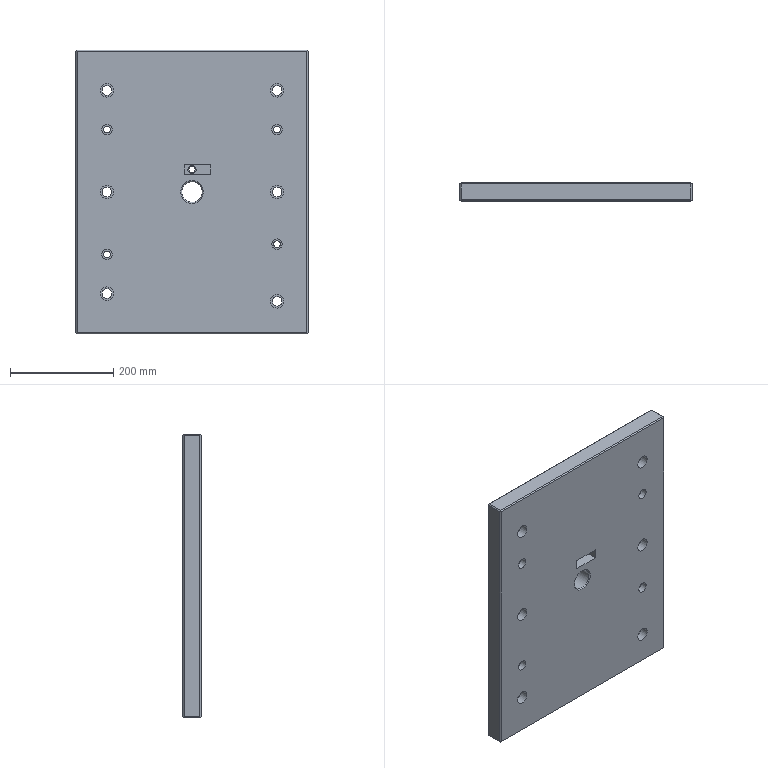Part | STEP file | BOTTOM-CLAMP-PLATE_id494_x_t | 1 solid | 59 faces | box 450 x 35 x 550 mm | volume 8473863 mm3 | plane 34 | cylinder 23 | cone 2 | commonest cylinder face diameters 18.5 x6 26 x6 13 x4 20 x4 12 x1 16 x1
STEP:
#1=CARTESIAN_POINT('',(-15.5,-265.5,53.));
#2=VERTEX_POINT('',#1);
#3=CARTESIAN_POINT('',(35.5,-265.5,53.));
#4=VERTEX_POINT('',#3);
#5=CARTESIAN_POINT('',(-15.,-265.5,53.));
#6=DIRECTION('',(1.,0.,0.));
#7=VECTOR('',#6,1.);
#8=LINE('',#5,#7);
#9=EDGE_CURVE('',#2,#4,#8,.T.);
#10=ORIENTED_EDGE('',*,*,#9,.T.);
#11=CARTESIAN_POINT('',(35.5,-290.5,53.));
#12=VERTEX_POINT('',#11);
#13=CARTESIAN_POINT('',(35.5,-290.5,53.));
#14=DIRECTION('',(0.,-1.,0.));
#15=VECTOR('',#14,1.);
#16=LINE('',#13,#15);
#17=EDGE_CURVE('',#4,#12,#16,.T.);
#18=ORIENTED_EDGE('',*,*,#17,.T.);
#19=CARTESIAN_POINT('',(-15.5,-290.5,53.));
#20=VERTEX_POINT('',#19);
#21=CARTESIAN_POINT('',(-200.,-290.5,53.));
#22=DIRECTION('',(1.,0.,0.));
#23=VECTOR('',#22,1.);
#24=LINE('',#21,#23);
#25=EDGE_CURVE('',#20,#12,#24,.T.);
#26=ORIENTED_EDGE('',*,*,#25,.F.);
#27=CARTESIAN_POINT('',(-15.5,-290.5,53.));
#28=DIRECTION('',(0.,1.,0.));
#29=VECTOR('',#28,1.);
#30=LINE('',#27,#29);
#31=EDGE_CURVE('',#20,#2,#30,.T.);
#32=ORIENTED_EDGE('',*,*,#31,.T.);
#33=EDGE_LOOP('',(#10,#18,#26,#32));
#34=FACE_OUTER_BOUND('',#33,.T.);
#35=CARTESIAN_POINT('',(35.5,-290.5,53.));
#36=DIRECTION('',(0.,0.,1.));
#37=DIRECTION('',(1.,0.,0.));
#38=AXIS2_PLACEMENT_3D('',#35,#36,#37);
#39=PLANE('',#38);
#40=ADVANCED_FACE('',(#34),#39,.F.);
#41=CARTESIAN_POINT('',(35.5,-265.5,34.));
#42=VERTEX_POINT('',#41);
#43=CARTESIAN_POINT('',(35.5,-265.5,52.5));
#44=DIRECTION('',(0.,0.,-1.));
#45=VECTOR('',#44,1.);
#46=LINE('',#43,#45);
#47=EDGE_CURVE('',#4,#42,#46,.T.);
#48=ORIENTED_EDGE('',*,*,#47,.T.);
#49=CARTESIAN_POINT('',(35.5,-290.5,34.));
#50=VERTEX_POINT('',#49);
#51=CARTESIAN_POINT('',(35.5,-290.5,34.));
#52=DIRECTION('',(0.,-1.,0.));
#53=VECTOR('',#52,1.);
#54=LINE('',#51,#53);
#55=EDGE_CURVE('',#42,#50,#54,.T.);
#56=ORIENTED_EDGE('',*,*,#55,.T.);
#57=CARTESIAN_POINT('',(35.5,-290.5,-275.));
#58=DIRECTION('',(0.,0.,-1.));
#59=VECTOR('',#58,1.);
#60=LINE('',#57,#59);
#61=EDGE_CURVE('',#12,#50,#60,.T.);
#62=ORIENTED_EDGE('',*,*,#61,.F.);
#63=ORIENTED_EDGE('',*,*,#17,.F.);
#64=EDGE_LOOP('',(#48,#56,#62,#63));
#65=FACE_OUTER_BOUND('',#64,.T.);
#66=CARTESIAN_POINT('',(35.5,-290.5,34.));
#67=DIRECTION('',(1.,0.,0.));
#68=DIRECTION('',(0.,0.,-1.));
#69=AXIS2_PLACEMENT_3D('',#66,#67,#68);
#70=PLANE('',#69);
#71=ADVANCED_FACE('',(#65),#70,.F.);
#72=CARTESIAN_POINT('',(-15.5,-265.5,34.));
#73=VERTEX_POINT('',#72);
#74=CARTESIAN_POINT('',(-15.,-265.5,34.));
#75=DIRECTION('',(-1.,0.,0.));
#76=VECTOR('',#75,1.);
#77=LINE('',#74,#76);
#78=EDGE_CURVE('',#42,#73,#77,.T.);
#79=ORIENTED_EDGE('',*,*,#78,.T.);
#80=CARTESIAN_POINT('',(-15.5,-290.5,34.));
#81=VERTEX_POINT('',#80);
#82=CARTESIAN_POINT('',(-15.5,-290.5,34.));
#83=DIRECTION('',(0.,-1.,0.));
#84=VECTOR('',#83,1.);
#85=LINE('',#82,#84);
#86=EDGE_CURVE('',#73,#81,#85,.T.);
#87=ORIENTED_EDGE('',*,*,#86,.T.);
#88=CARTESIAN_POINT('',(-200.,-290.5,34.));
#89=DIRECTION('',(-1.,0.,0.));
#90=VECTOR('',#89,1.);
#91=LINE('',#88,#90);
#92=EDGE_CURVE('',#50,#81,#91,.T.);
#93=ORIENTED_EDGE('',*,*,#92,.F.);
#94=ORIENTED_EDGE('',*,*,#55,.F.);
#95=EDGE_LOOP('',(#79,#87,#93,#94));
#96=FACE_OUTER_BOUND('',#95,.T.);
#97=CARTESIAN_POINT('',(-15.5,-290.5,34.));
#98=DIRECTION('',(0.,0.,-1.));
#99=DIRECTION('',(-1.,0.,0.));
#100=AXIS2_PLACEMENT_3D('',#97,#98,#99);
#101=PLANE('',#100);
#102=ADVANCED_FACE('',(#96),#101,.F.);
#103=CARTESIAN_POINT('',(-15.5,-265.5,52.5));
#104=DIRECTION('',(0.,0.,1.));
#105=VECTOR('',#104,1.);
#106=LINE('',#103,#105);
#107=EDGE_CURVE('',#73,#2,#106,.T.);
#108=ORIENTED_EDGE('',*,*,#107,.T.);
#109=ORIENTED_EDGE('',*,*,#31,.F.);
#110=CARTESIAN_POINT('',(-15.5,-290.5,-275.));
#111=DIRECTION('',(0.,0.,1.));
#112=VECTOR('',#111,1.);
#113=LINE('',#110,#112);
#114=EDGE_CURVE('',#81,#20,#113,.T.);
#115=ORIENTED_EDGE('',*,*,#114,.F.);
#116=ORIENTED_EDGE('',*,*,#86,.F.);
#117=EDGE_LOOP('',(#108,#109,#115,#116));
#118=FACE_OUTER_BOUND('',#117,.T.);
#119=CARTESIAN_POINT('',(-15.5,-290.5,53.));
#120=DIRECTION('',(-1.,0.,0.));
#121=DIRECTION('',(0.,0.,1.));
#122=AXIS2_PLACEMENT_3D('',#119,#120,#121);
#123=PLANE('',#122);
#124=ADVANCED_FACE('',(#118),#123,.F.);
#125=ORIENTED_EDGE('',*,*,#114,.T.);
#126=ORIENTED_EDGE('',*,*,#25,.T.);
#127=ORIENTED_EDGE('',*,*,#61,.T.);
#128=ORIENTED_EDGE('',*,*,#92,.T.);
#129=EDGE_LOOP('',(#125,#126,#127,#128));
#130=FACE_BOUND('',#129,.T.);
#131=CARTESIAN_POINT('',(-165.,-290.5,111.));
#132=VERTEX_POINT('',#131);
#133=CARTESIAN_POINT('',(-165.,-290.5,121.));
#134=DIRECTION('',(0.,1.,0.));
#135=DIRECTION('',(0.,0.,-1.));
#136=AXIS2_PLACEMENT_3D('',#133,#134,#135);
#137=CIRCLE('',#136,10.);
#138=EDGE_CURVE('',#132,#132,#137,.T.);
#139=ORIENTED_EDGE('',*,*,#138,.T.);
#140=EDGE_LOOP('',(#139));
#141=FACE_BOUND('',#140,.T.);
#142=CARTESIAN_POINT('',(165.,-290.5,111.));
#143=VERTEX_POINT('',#142);
#144=CARTESIAN_POINT('',(165.,-290.5,121.));
#145=DIRECTION('',(0.,1.,0.));
#146=DIRECTION('',(0.,0.,-1.));
#147=AXIS2_PLACEMENT_3D('',#144,#145,#146);
#148=CIRCLE('',#147,10.);
#149=EDGE_CURVE('',#143,#143,#148,.T.);
#150=ORIENTED_EDGE('',*,*,#149,.T.);
#151=EDGE_LOOP('',(#150));
#152=FACE_BOUND('',#151,.T.);
#153=CARTESIAN_POINT('',(165.,-290.5,-111.));
#154=VERTEX_POINT('',#153);
#155=CARTESIAN_POINT('',(165.,-290.5,-101.));
#156=DIRECTION('',(0.,1.,0.));
#157=DIRECTION('',(0.,0.,-1.));
#158=AXIS2_PLACEMENT_3D('',#155,#156,#157);
#159=CIRCLE('',#158,10.);
#160=EDGE_CURVE('',#154,#154,#159,.T.);
#161=ORIENTED_EDGE('',*,*,#160,.T.);
#162=EDGE_LOOP('',(#161));
#163=FACE_BOUND('',#162,.T.);
#164=CARTESIAN_POINT('',(-165.,-290.5,-131.));
#165=VERTEX_POINT('',#164);
#166=CARTESIAN_POINT('',(-165.,-290.5,-121.));
#167=DIRECTION('',(0.,1.,0.));
#168=DIRECTION('',(0.,0.,-1.));
#169=AXIS2_PLACEMENT_3D('',#166,#167,#168);
#170=CIRCLE('',#169,10.);
#171=EDGE_CURVE('',#165,#165,#170,.T.);
#172=ORIENTED_EDGE('',*,*,#171,.T.);
#173=EDGE_LOOP('',(#172));
#174=FACE_BOUND('',#173,.T.);
#175=CARTESIAN_POINT('',(165.,-290.5,-13.));
#176=VERTEX_POINT('',#175);
#177=CARTESIAN_POINT('',(165.,-290.5,0.));
#178=DIRECTION('',(0.,1.,0.));
#179=DIRECTION('',(0.,0.,-1.));
#180=AXIS2_PLACEMENT_3D('',#177,#178,#179);
#181=CIRCLE('',#180,13.);
#182=EDGE_CURVE('',#176,#176,#181,.T.);
#183=ORIENTED_EDGE('',*,*,#182,.T.);
#184=EDGE_LOOP('',(#183));
#185=FACE_BOUND('',#184,.T.);
#186=CARTESIAN_POINT('',(-165.,-290.5,-13.));
#187=VERTEX_POINT('',#186);
#188=CARTESIAN_POINT('',(-165.,-290.5,0.));
#189=DIRECTION('',(0.,1.,0.));
#190=DIRECTION('',(0.,0.,-1.));
#191=AXIS2_PLACEMENT_3D('',#188,#189,#190);
#192=CIRCLE('',#191,13.);
#193=EDGE_CURVE('',#187,#187,#192,.T.);
#194=ORIENTED_EDGE('',*,*,#193,.T.);
#195=EDGE_LOOP('',(#194));
#196=FACE_BOUND('',#195,.T.);
#197=CARTESIAN_POINT('',(-165.,-290.5,184.));
#198=VERTEX_POINT('',#197);
#199=CARTESIAN_POINT('',(-165.,-290.5,197.));
#200=DIRECTION('',(0.,1.,0.));
#201=DIRECTION('',(0.,0.,-1.));
#202=AXIS2_PLACEMENT_3D('',#199,#200,#201);
#203=CIRCLE('',#202,13.);
#204=EDGE_CURVE('',#198,#198,#203,.T.);
#205=ORIENTED_EDGE('',*,*,#204,.T.);
#206=EDGE_LOOP('',(#205));
#207=FACE_BOUND('',#206,.T.);
#208=CARTESIAN_POINT('',(165.,-290.5,184.));
#209=VERTEX_POINT('',#208);
#210=CARTESIAN_POINT('',(165.,-290.5,197.));
#211=DIRECTION('',(0.,1.,0.));
#212=DIRECTION('',(0.,0.,-1.));
#213=AXIS2_PLACEMENT_3D('',#210,#211,#212);
#214=CIRCLE('',#213,13.);
#215=EDGE_CURVE('',#209,#209,#214,.T.);
#216=ORIENTED_EDGE('',*,*,#215,.T.);
#217=EDGE_LOOP('',(#216));
#218=FACE_BOUND('',#217,.T.);
#219=CARTESIAN_POINT('',(165.,-290.5,-225.));
#220=VERTEX_POINT('',#219);
#221=CARTESIAN_POINT('',(165.,-290.5,-212.));
#222=DIRECTION('',(0.,1.,0.));
#223=DIRECTION('',(0.,0.,-1.));
#224=AXIS2_PLACEMENT_3D('',#221,#222,#223);
#225=CIRCLE('',#224,13.);
#226=EDGE_CURVE('',#220,#220,#225,.T.);
#227=ORIENTED_EDGE('',*,*,#226,.T.);
#228=EDGE_LOOP('',(#227));
#229=FACE_BOUND('',#228,.T.);
#230=CARTESIAN_POINT('',(-165.,-290.5,-210.));
#231=VERTEX_POINT('',#230);
#232=CARTESIAN_POINT('',(-165.,-290.5,-197.));
#233=DIRECTION('',(0.,1.,0.));
#234=DIRECTION('',(0.,0.,-1.));
#235=AXIS2_PLACEMENT_3D('',#232,#233,#234);
#236=CIRCLE('',#235,13.);
#237=EDGE_CURVE('',#231,#231,#236,.T.);
#238=ORIENTED_EDGE('',*,*,#237,.T.);
#239=EDGE_LOOP('',(#238));
#240=FACE_BOUND('',#239,.T.);
#241=CARTESIAN_POINT('',(0.,-290.5,-22.));
#242=VERTEX_POINT('',#241);
#243=CARTESIAN_POINT('',(0.,-290.5,0.));
#244=DIRECTION('',(0.,1.,0.));
#245=DIRECTION('',(0.,0.,-1.));
#246=AXIS2_PLACEMENT_3D('',#243,#244,#245);
#247=CIRCLE('',#246,22.);
#248=EDGE_CURVE('',#242,#242,#247,.T.);
#249=ORIENTED_EDGE('',*,*,#248,.T.);
#250=EDGE_LOOP('',(#249));
#251=FACE_BOUND('',#250,.T.);
#252=CARTESIAN_POINT('',(-223.,-290.5,-273.));
#253=VERTEX_POINT('',#252);
#254=CARTESIAN_POINT('',(223.,-290.5,-273.));
#255=VERTEX_POINT('',#254);
#256=CARTESIAN_POINT('',(-223.,-290.5,-273.));
#257=DIRECTION('',(1.,0.,0.));
#258=VECTOR('',#257,1.);
#259=LINE('',#256,#258);
#260=EDGE_CURVE('',#253,#255,#259,.T.);
#261=ORIENTED_EDGE('',*,*,#260,.T.);
#262=CARTESIAN_POINT('',(223.,-290.5,273.));
#263=VERTEX_POINT('',#262);
#264=CARTESIAN_POINT('',(223.,-290.5,-275.));
#265=DIRECTION('',(0.,0.,1.));
#266=VECTOR('',#265,1.);
#267=LINE('',#264,#266);
#268=EDGE_CURVE('',#255,#263,#267,.T.);
#269=ORIENTED_EDGE('',*,*,#268,.T.);
#270=CARTESIAN_POINT('',(-223.,-290.5,273.));
#271=VERTEX_POINT('',#270);
#272=CARTESIAN_POINT('',(223.,-290.5,273.));
#273=DIRECTION('',(-1.,0.,0.));
#274=VECTOR('',#273,1.);
#275=LINE('',#272,#274);
#276=EDGE_CURVE('',#263,#271,#275,.T.);
#277=ORIENTED_EDGE('',*,*,#276,.T.);
#278=CARTESIAN_POINT('',(-223.,-290.5,273.));
#279=DIRECTION('',(0.,0.,-1.));
#280=VECTOR('',#279,1.);
#281=LINE('',#278,#280);
#282=EDGE_CURVE('',#271,#253,#281,.T.);
#283=ORIENTED_EDGE('',*,*,#282,.T.);
#284=EDGE_LOOP('',(#261,#269,#277,#283));
#285=FACE_BOUND('',#284,.T.);
#286=CARTESIAN_POINT('',(-200.,-290.5,-275.));
#287=DIRECTION('',(0.,-1.,0.));
#288=DIRECTION('',(0.,0.,-1.));
#289=AXIS2_PLACEMENT_3D('',#286,#287,#288);
#290=PLANE('',#289);
#291=ADVANCED_FACE('',(#130,#141,#152,#163,#174,#185,#196,#207,#218,#229,#240,#251,#285),#290,.T.);
#292=CARTESIAN_POINT('',(0.,-265.5,35.5));
#293=VERTEX_POINT('',#292);
#294=CARTESIAN_POINT('',(0.,-265.5,43.5));
#295=DIRECTION('',(0.,1.,0.));
#296=DIRECTION('',(0.,0.,-1.));
#297=AXIS2_PLACEMENT_3D('',#294,#295,#296);
#298=CIRCLE('',#297,8.);
#299=EDGE_CURVE('',#293,#293,#298,.T.);
#300=ORIENTED_EDGE('',*,*,#299,.T.);
#301=EDGE_LOOP('',(#300));
#302=FACE_BOUND('',#301,.T.);
#303=ORIENTED_EDGE('',*,*,#78,.F.);
#304=ORIENTED_EDGE('',*,*,#47,.F.);
#305=ORIENTED_EDGE('',*,*,#9,.F.);
#306=ORIENTED_EDGE('',*,*,#107,.F.);
#307=EDGE_LOOP('',(#303,#304,#305,#306));
#308=FACE_BOUND('',#307,.T.);
#309=CARTESIAN_POINT('',(-15.,-265.5,52.5));
#310=DIRECTION('',(0.,1.,0.));
#311=DIRECTION('',(0.,0.,1.));
#312=AXIS2_PLACEMENT_3D('',#309,#310,#311);
#313=PLANE('',#312);
#314=ADVANCED_FACE('',(#302,#308),#313,.F.);
#315=CARTESIAN_POINT('',(225.,-288.5,-273.));
#316=VERTEX_POINT('',#315);
#317=CARTESIAN_POINT('',(224.,-289.5,-274.));
#318=VERTEX_POINT('',#317);
#319=CARTESIAN_POINT('',(225.,-288.5,-273.));
#320=DIRECTION('',(-0.5774,-0.5774,-0.5774));
#321=VECTOR('',#320,1.);
#322=LINE('',#319,#321);
#323=EDGE_CURVE('',#316,#318,#322,.T.);
#324=ORIENTED_EDGE('',*,*,#323,.F.);
#325=CARTESIAN_POINT('',(225.,-288.5,273.));
#326=VERTEX_POINT('',#325);
#327=CARTESIAN_POINT('',(225.,-288.5,-275.));
#328=DIRECTION('',(0.,0.,-1.));
#329=VECTOR('',#328,1.);
#330=LINE('',#327,#329);
#331=EDGE_CURVE('',#326,#316,#330,.T.);
#332=ORIENTED_EDGE('',*,*,#331,.F.);
#333=CARTESIAN_POINT('',(224.,-289.5,274.));
#334=VERTEX_POINT('',#333);
#335=CARTESIAN_POINT('',(224.,-289.5,274.));
#336=DIRECTION('',(0.5774,0.5774,-0.5774));
#337=VECTOR('',#336,1.);
#338=LINE('',#335,#337);
#339=EDGE_CURVE('',#334,#326,#338,.T.);
#340=ORIENTED_EDGE('',*,*,#339,.F.);
#341=CARTESIAN_POINT('',(224.,-289.5,274.));
#342=DIRECTION('',(-0.5774,-0.5774,-0.5774));
#343=VECTOR('',#342,1.);
#344=LINE('',#341,#343);
#345=EDGE_CURVE('',#334,#263,#344,.T.);
#346=ORIENTED_EDGE('',*,*,#345,.T.);
#347=ORIENTED_EDGE('',*,*,#268,.F.);
#348=CARTESIAN_POINT('',(223.,-290.5,-273.));
#349=DIRECTION('',(0.5774,0.5774,-0.5774));
#350=VECTOR('',#349,1.);
#351=LINE('',#348,#350);
#352=EDGE_CURVE('',#255,#318,#351,.T.);
#353=ORIENTED_EDGE('',*,*,#352,.T.);
#354=EDGE_LOOP('',(#324,#332,#340,#346,#347,#353));
#355=FACE_OUTER_BOUND('',#354,.T.);
#356=CARTESIAN_POINT('',(223.,-290.5,-275.));
#357=DIRECTION('',(-0.7071,0.7071,0.));
#358=DIRECTION('',(-0.7071,-0.7071,0.));
#359=AXIS2_PLACEMENT_3D('',#356,#357,#358);
#360=PLANE('',#359);
#361=ADVANCED_FACE('',(#355),#360,.F.);
#362=CARTESIAN_POINT('',(223.,-288.5,275.));
#363=VERTEX_POINT('',#362);
#364=CARTESIAN_POINT('',(223.,-288.5,275.));
#365=DIRECTION('',(0.5774,-0.5774,-0.5774));
#366=VECTOR('',#365,1.);
#367=LINE('',#364,#366);
#368=EDGE_CURVE('',#363,#334,#367,.T.);
#369=ORIENTED_EDGE('',*,*,#368,.F.);
#370=CARTESIAN_POINT('',(-223.,-288.5,275.));
#371=VERTEX_POINT('',#370);
#372=CARTESIAN_POINT('',(225.,-288.5,275.));
#373=DIRECTION('',(1.,0.,0.));
#374=VECTOR('',#373,1.);
#375=LINE('',#372,#374);
#376=EDGE_CURVE('',#371,#363,#375,.T.);
#377=ORIENTED_EDGE('',*,*,#376,.F.);
#378=CARTESIAN_POINT('',(-224.,-289.5,274.));
#379=VERTEX_POINT('',#378);
#380=CARTESIAN_POINT('',(-224.,-289.5,274.));
#381=DIRECTION('',(0.5774,0.5774,0.5774));
#382=VECTOR('',#381,1.);
#383=LINE('',#380,#382);
#384=EDGE_CURVE('',#379,#371,#383,.T.);
#385=ORIENTED_EDGE('',*,*,#384,.F.);
#386=CARTESIAN_POINT('',(-224.,-289.5,274.));
#387=DIRECTION('',(0.5774,-0.5774,-0.5774));
#388=VECTOR('',#387,1.);
#389=LINE('',#386,#388);
#390=EDGE_CURVE('',#379,#271,#389,.T.);
#391=ORIENTED_EDGE('',*,*,#390,.T.);
#392=ORIENTED_EDGE('',*,*,#276,.F.);
#393=ORIENTED_EDGE('',*,*,#345,.F.);
#394=EDGE_LOOP('',(#369,#377,#385,#391,#392,#393));
#395=FACE_OUTER_BOUND('',#394,.T.);
#396=CARTESIAN_POINT('',(223.,-290.5,273.));
#397=DIRECTION('',(0.,0.7071,-0.7071));
#398=DIRECTION('',(0.,0.7071,0.7071));
#399=AXIS2_PLACEMENT_3D('',#396,#397,#398);
#400=PLANE('',#399);
#401=ADVANCED_FACE('',(#395),#400,.F.);
#402=CARTESIAN_POINT('',(224.,-256.5,274.));
#403=VERTEX_POINT('',#402);
#404=CARTESIAN_POINT('',(223.,-257.5,275.));
#405=VERTEX_POINT('',#404);
#406=CARTESIAN_POINT('',(224.,-256.5,274.));
#407=DIRECTION('',(-0.5774,-0.5774,0.5774));
#408=VECTOR('',#407,1.);
#409=LINE('',#406,#408);
#410=EDGE_CURVE('',#403,#405,#409,.T.);
#411=ORIENTED_EDGE('',*,*,#410,.T.);
#412=CARTESIAN_POINT('',(223.,-255.5,275.));
#413=DIRECTION('',(0.,1.,0.));
#414=VECTOR('',#413,1.);
#415=LINE('',#412,#414);
#416=EDGE_CURVE('',#363,#405,#415,.T.);
#417=ORIENTED_EDGE('',*,*,#416,.F.);
#418=ORIENTED_EDGE('',*,*,#368,.T.);
#419=ORIENTED_EDGE('',*,*,#339,.T.);
#420=CARTESIAN_POINT('',(225.,-257.5,273.));
#421=VERTEX_POINT('',#420);
#422=CARTESIAN_POINT('',(225.,-255.5,273.));
#423=DIRECTION('',(0.,-1.,0.));
#424=VECTOR('',#423,1.);
#425=LINE('',#422,#424);
#426=EDGE_CURVE('',#421,#326,#425,.T.);
#427=ORIENTED_EDGE('',*,*,#426,.F.);
#428=CARTESIAN_POINT('',(225.,-257.5,273.));
#429=DIRECTION('',(-0.5774,0.5774,0.5774));
#430=VECTOR('',#429,1.);
#431=LINE('',#428,#430);
#432=EDGE_CURVE('',#421,#403,#431,.T.);
#433=ORIENTED_EDGE('',*,*,#432,.T.);
#434=EDGE_LOOP('',(#411,#417,#418,#419,#427,#433));
#435=FACE_OUTER_BOUND('',#434,.T.);
#436=CARTESIAN_POINT('',(223.,-255.5,275.));
#437=DIRECTION('',(0.7071,0.,0.7071));
#438=DIRECTION('',(0.7071,0.,-0.7071));
#439=AXIS2_PLACEMENT_3D('',#436,#437,#438);
#440=PLANE('',#439);
#441=ADVANCED_FACE('',(#435),#440,.T.);
#442=CARTESIAN_POINT('',(-225.,-288.5,273.));
#443=VERTEX_POINT('',#442);
#444=CARTESIAN_POINT('',(-225.,-288.5,273.));
#445=DIRECTION('',(0.5774,-0.5774,0.5774));
#446=VECTOR('',#445,1.);
#447=LINE('',#444,#446);
#448=EDGE_CURVE('',#443,#379,#447,.T.);
#449=ORIENTED_EDGE('',*,*,#448,.F.);
#450=CARTESIAN_POINT('',(-225.,-288.5,-273.));
#451=VERTEX_POINT('',#450);
#452=CARTESIAN_POINT('',(-225.,-288.5,275.));
#453=DIRECTION('',(0.,0.,1.));
#454=VECTOR('',#453,1.);
#455=LINE('',#452,#454);
#456=EDGE_CURVE('',#451,#443,#455,.T.);
#457=ORIENTED_EDGE('',*,*,#456,.F.);
#458=CARTESIAN_POINT('',(-224.,-289.5,-274.));
#459=VERTEX_POINT('',#458);
#460=CARTESIAN_POINT('',(-224.,-289.5,-274.));
#461=DIRECTION('',(-0.5774,0.5774,0.5774));
#462=VECTOR('',#461,1.);
#463=LINE('',#460,#462);
#464=EDGE_CURVE('',#459,#451,#463,.T.);
#465=ORIENTED_EDGE('',*,*,#464,.F.);
#466=CARTESIAN_POINT('',(-224.,-289.5,-274.));
#467=DIRECTION('',(0.5774,-0.5774,0.5774));
#468=VECTOR('',#467,1.);
#469=LINE('',#466,#468);
#470=EDGE_CURVE('',#459,#253,#469,.T.);
#471=ORIENTED_EDGE('',*,*,#470,.T.);
#472=ORIENTED_EDGE('',*,*,#282,.F.);
#473=ORIENTED_EDGE('',*,*,#390,.F.);
#474=EDGE_LOOP('',(#449,#457,#465,#471,#472,#473));
#475=FACE_OUTER_BOUND('',#474,.T.);
#476=CARTESIAN_POINT('',(-223.,-290.5,273.));
#477=DIRECTION('',(0.7071,0.7071,0.));
#478=DIRECTION('',(-0.7071,0.7071,0.));
#479=AXIS2_PLACEMENT_3D('',#476,#477,#478);
#480=PLANE('',#479);
#481=ADVANCED_FACE('',(#475),#480,.F.);
#482=CARTESIAN_POINT('',(-224.,-256.5,274.));
#483=VERTEX_POINT('',#482);
#484=CARTESIAN_POINT('',(-225.,-257.5,273.));
#485=VERTEX_POINT('',#484);
#486=CARTESIAN_POINT('',(-224.,-256.5,274.));
#487=DIRECTION('',(-0.5774,-0.5774,-0.5774));
#488=VECTOR('',#487,1.);
#489=LINE('',#486,#488);
#490=EDGE_CURVE('',#483,#485,#489,.T.);
#491=ORIENTED_EDGE('',*,*,#490,.T.);
#492=CARTESIAN_POINT('',(-225.,-255.5,273.));
#493=DIRECTION('',(0.,1.,0.));
#494=VECTOR('',#493,1.);
#495=LINE('',#492,#494);
#496=EDGE_CURVE('',#443,#485,#495,.T.);
#497=ORIENTED_EDGE('',*,*,#496,.F.);
#498=ORIENTED_EDGE('',*,*,#448,.T.);
#499=ORIENTED_EDGE('',*,*,#384,.T.);
#500=CARTESIAN_POINT('',(-223.,-257.5,275.));
#501=VERTEX_POINT('',#500);
#502=CARTESIAN_POINT('',(-223.,-255.5,275.));
#503=DIRECTION('',(0.,-1.,0.));
#504=VECTOR('',#503,1.);
#505=LINE('',#502,#504);
#506=EDGE_CURVE('',#501,#371,#505,.T.);
#507=ORIENTED_EDGE('',*,*,#506,.F.);
#508=CARTESIAN_POINT('',(-223.,-257.5,275.));
#509=DIRECTION('',(-0.5774,0.5774,-0.5774));
#510=VECTOR('',#509,1.);
#511=LINE('',#508,#510);
#512=EDGE_CURVE('',#501,#483,#511,.T.);
#513=ORIENTED_EDGE('',*,*,#512,.T.);
#514=EDGE_LOOP('',(#491,#497,#498,#499,#507,#513));
#515=FACE_OUTER_BOUND('',#514,.T.);
#516=CARTESIAN_POINT('',(-225.,-255.5,273.));
#517=DIRECTION('',(-0.7071,0.,0.7071));
#518=DIRECTION('',(0.7071,0.,0.7071));
#519=AXIS2_PLACEMENT_3D('',#516,#517,#518);
#520=PLANE('',#519);
#521=ADVANCED_FACE('',(#515),#520,.T.);
#522=CARTESIAN_POINT('',(224.,-256.5,-274.));
#523=VERTEX_POINT('',#522);
#524=CARTESIAN_POINT('',(225.,-257.5,-273.));
#525=VERTEX_POINT('',#524);
#526=CARTESIAN_POINT('',(224.,-256.5,-274.));
#527=DIRECTION('',(0.5774,-0.5774,0.5774));
#528=VECTOR('',#527,1.);
#529=LINE('',#526,#528);
#530=EDGE_CURVE('',#523,#525,#529,.T.);
#531=ORIENTED_EDGE('',*,*,#530,.T.);
#532=CARTESIAN_POINT('',(225.,-255.5,-273.));
#533=DIRECTION('',(0.,1.,0.));
#534=VECTOR('',#533,1.);
#535=LINE('',#532,#534);
#536=EDGE_CURVE('',#316,#525,#535,.T.);
#537=ORIENTED_EDGE('',*,*,#536,.F.);
#538=ORIENTED_EDGE('',*,*,#323,.T.);
#539=CARTESIAN_POINT('',(223.,-288.5,-275.));
#540=VERTEX_POINT('',#539);
#541=CARTESIAN_POINT('',(224.,-289.5,-274.));
#542=DIRECTION('',(-0.5774,0.5774,-0.5774));
#543=VECTOR('',#542,1.);
#544=LINE('',#541,#543);
#545=EDGE_CURVE('',#318,#540,#544,.T.);
#546=ORIENTED_EDGE('',*,*,#545,.T.);
#547=CARTESIAN_POINT('',(223.,-257.5,-275.));
#548=VERTEX_POINT('',#547);
#549=CARTESIAN_POINT('',(223.,-255.5,-275.));
#550=DIRECTION('',(0.,-1.,0.));
#551=VECTOR('',#550,1.);
#552=LINE('',#549,#551);
#553=EDGE_CURVE('',#548,#540,#552,.T.);
#554=ORIENTED_EDGE('',*,*,#553,.F.);
#555=CARTESIAN_POINT('',(223.,-257.5,-275.));
#556=DIRECTION('',(0.5774,0.5774,0.5774));
#557=VECTOR('',#556,1.);
#558=LINE('',#555,#557);
#559=EDGE_CURVE('',#548,#523,#558,.T.);
#560=ORIENTED_EDGE('',*,*,#559,.T.);
#561=EDGE_LOOP('',(#531,#537,#538,#546,#554,#560));
#562=FACE_OUTER_BOUND('',#561,.T.);
#563=CARTESIAN_POINT('',(225.,-257.5,-273.));
#564=DIRECTION('',(0.7071,0.,-0.7071));
#565=DIRECTION('',(-0.7071,0.,-0.7071));
#566=AXIS2_PLACEMENT_3D('',#563,#564,#565);
#567=PLANE('',#566);
#568=ADVANCED_FACE('',(#562),#567,.T.);
#569=CARTESIAN_POINT('',(-223.,-288.5,-275.));
#570=VERTEX_POINT('',#569);
#571=CARTESIAN_POINT('',(-223.,-288.5,-275.));
#572=DIRECTION('',(-0.5774,-0.5774,0.5774));
#573=VECTOR('',#572,1.);
#574=LINE('',#571,#573);
#575=EDGE_CURVE('',#570,#459,#574,.T.);
#576=ORIENTED_EDGE('',*,*,#575,.F.);
#577=CARTESIAN_POINT('',(-225.,-288.5,-275.));
#578=DIRECTION('',(-1.,0.,0.));
#579=VECTOR('',#578,1.);
#580=LINE('',#577,#579);
#581=EDGE_CURVE('',#540,#570,#580,.T.);
#582=ORIENTED_EDGE('',*,*,#581,.F.);
#583=ORIENTED_EDGE('',*,*,#545,.F.);
#584=ORIENTED_EDGE('',*,*,#352,.F.);
#585=ORIENTED_EDGE('',*,*,#260,.F.);
#586=ORIENTED_EDGE('',*,*,#470,.F.);
#587=EDGE_LOOP('',(#576,#582,#583,#584,#585,#586));
#588=FACE_OUTER_BOUND('',#587,.T.);
#589=CARTESIAN_POINT('',(-223.,-290.5,-273.));
#590=DIRECTION('',(0.,0.7071,0.7071));
#591=DIRECTION('',(0.,-0.7071,0.7071));
#592=AXIS2_PLACEMENT_3D('',#589,#590,#591);
#593=PLANE('',#592);
#594=ADVANCED_FACE('',(#588),#593,.F.);
#595=CARTESIAN_POINT('',(-224.,-256.5,-274.));
#596=VERTEX_POINT('',#595);
#597=CARTESIAN_POINT('',(-223.,-257.5,-275.));
#598=VERTEX_POINT('',#597);
#599=CARTESIAN_POINT('',(-224.,-256.5,-274.));
#600=DIRECTION('',(0.5774,-0.5774,-0.5774));
#601=VECTOR('',#600,1.);
#602=LINE('',#599,#601);
#603=EDGE_CURVE('',#596,#598,#602,.T.);
#604=ORIENTED_EDGE('',*,*,#603,.T.);
#605=CARTESIAN_POINT('',(-223.,-255.5,-275.));
#606=DIRECTION('',(0.,1.,0.));
#607=VECTOR('',#606,1.);
#608=LINE('',#605,#607);
#609=EDGE_CURVE('',#570,#598,#608,.T.);
#610=ORIENTED_EDGE('',*,*,#609,.F.);
#611=ORIENTED_EDGE('',*,*,#575,.T.);
#612=ORIENTED_EDGE('',*,*,#464,.T.);
#613=CARTESIAN_POINT('',(-225.,-257.5,-273.));
#614=VERTEX_POINT('',#613);
#615=CARTESIAN_POINT('',(-225.,-255.5,-273.));
#616=DIRECTION('',(0.,-1.,0.));
#617=VECTOR('',#616,1.);
#618=LINE('',#615,#617);
#619=EDGE_CURVE('',#614,#451,#618,.T.);
#620=ORIENTED_EDGE('',*,*,#619,.F.);
#621=CARTESIAN_POINT('',(-225.,-257.5,-273.));
#622=DIRECTION('',(0.5774,0.5774,-0.5774));
#623=VECTOR('',#622,1.);
#624=LINE('',#621,#623);
#625=EDGE_CURVE('',#614,#596,#624,.T.);
#626=ORIENTED_EDGE('',*,*,#625,.T.);
#627=EDGE_LOOP('',(#604,#610,#611,#612,#620,#626));
#628=FACE_OUTER_BOUND('',#627,.T.);
#629=CARTESIAN_POINT('',(-223.,-257.5,-275.));
#630=DIRECTION('',(-0.7071,0.,-0.7071));
#631=DIRECTION('',(-0.7071,0.,0.7071));
#632=AXIS2_PLACEMENT_3D('',#629,#630,#631);
#633=PLANE('',#632);
#634=ADVANCED_FACE('',(#628),#633,.T.);
#635=CARTESIAN_POINT('',(0.,-288.5,20.));
#636=VERTEX_POINT('',#635);
#637=CARTESIAN_POINT('',(0.,-288.5,0.));
#638=DIRECTION('',(0.,1.,0.));
#639=DIRECTION('',(0.,0.,1.));
#640=AXIS2_PLACEMENT_3D('',#637,#638,#639);
#641=CIRCLE('',#640,20.);
#642=EDGE_CURVE('',#636,#636,#641,.T.);
#643=ORIENTED_EDGE('',*,*,#642,.T.);
#644=EDGE_LOOP('',(#643));
#645=FACE_BOUND('',#644,.T.);
#646=ORIENTED_EDGE('',*,*,#248,.F.);
#647=EDGE_LOOP('',(#646));
#648=FACE_BOUND('',#647,.T.);
#649=CARTESIAN_POINT('',(0.,-290.5,0.));
#650=DIRECTION('',(0.,-1.,0.));
#651=DIRECTION('',(0.,0.,-1.));
#652=AXIS2_PLACEMENT_3D('',#649,#650,#651);
#653=CONICAL_SURFACE('',#652,22.,45.);
#654=ADVANCED_FACE('',(#645,#648),#653,.F.);
#655=CARTESIAN_POINT('',(165.,-274.,-225.));
#656=VERTEX_POINT('',#655);
#657=CARTESIAN_POINT('',(165.,-274.,-212.));
#658=DIRECTION('',(0.,-1.,0.));
#659=DIRECTION('',(0.,0.,-1.));
#660=AXIS2_PLACEMENT_3D('',#657,#658,#659);
#661=CIRCLE('',#660,13.);
#662=EDGE_CURVE('',#656,#656,#661,.T.);
#663=ORIENTED_EDGE('',*,*,#662,.F.);
#664=EDGE_LOOP('',(#663));
#665=FACE_BOUND('',#664,.T.);
#666=ORIENTED_EDGE('',*,*,#226,.F.);
#667=EDGE_LOOP('',(#666));
#668=FACE_BOUND('',#667,.T.);
#669=CARTESIAN_POINT('',(165.,-290.5,-212.));
#670=DIRECTION('',(0.,-1.,0.));
#671=DIRECTION('',(0.,0.,-1.));
#672=AXIS2_PLACEMENT_3D('',#669,#670,#671);
#673=CYLINDRICAL_SURFACE('',#672,13.);
#674=ADVANCED_FACE('',(#665,#668),#673,.F.);
#675=CARTESIAN_POINT('',(165.,-277.5,-111.));
#676=VERTEX_POINT('',#675);
#677=CARTESIAN_POINT('',(165.,-277.5,-101.));
#678=DIRECTION('',(0.,-1.,0.));
#679=DIRECTION('',(0.,0.,-1.));
#680=AXIS2_PLACEMENT_3D('',#677,#678,#679);
#681=CIRCLE('',#680,10.);
#682=EDGE_CURVE('',#676,#676,#681,.T.);
#683=ORIENTED_EDGE('',*,*,#682,.F.);
#684=EDGE_LOOP('',(#683));
#685=FACE_BOUND('',#684,.T.);
#686=ORIENTED_EDGE('',*,*,#160,.F.);
#687=EDGE_LOOP('',(#686));
#688=FACE_BOUND('',#687,.T.);
#689=CARTESIAN_POINT('',(165.,-290.5,-101.));
#690=DIRECTION('',(0.,-1.,0.));
#691=DIRECTION('',(0.,0.,-1.));
#692=AXIS2_PLACEMENT_3D('',#689,#690,#691);
#693=CYLINDRICAL_SURFACE('',#692,10.);
#694=ADVANCED_FACE('',(#685,#688),#693,.F.);
#695=CARTESIAN_POINT('',(165.,-274.,-13.));
#696=VERTEX_POINT('',#695);
#697=CARTESIAN_POINT('',(165.,-274.,0.));
#698=DIRECTION('',(0.,-1.,0.));
#699=DIRECTION('',(0.,0.,-1.));
#700=AXIS2_PLACEMENT_3D('',#697,#698,#699);
#701=CIRCLE('',#700,13.);
#702=EDGE_CURVE('',#696,#696,#701,.T.);
#703=ORIENTED_EDGE('',*,*,#702,.F.);
#704=EDGE_LOOP('',(#703));
#705=FACE_BOUND('',#704,.T.);
#706=ORIENTED_EDGE('',*,*,#182,.F.);
#707=EDGE_LOOP('',(#706));
#708=FACE_BOUND('',#707,.T.);
#709=CARTESIAN_POINT('',(165.,-290.5,0.));
#710=DIRECTION('',(0.,-1.,0.));
#711=DIRECTION('',(0.,0.,-1.));
#712=AXIS2_PLACEMENT_3D('',#709,#710,#711);
#713=CYLINDRICAL_SURFACE('',#712,13.);
#714=ADVANCED_FACE('',(#705,#708),#713,.F.);
#715=CARTESIAN_POINT('',(165.,-277.5,111.));
#716=VERTEX_POINT('',#715);
#717=CARTESIAN_POINT('',(165.,-277.5,121.));
#718=DIRECTION('',(0.,-1.,0.));
#719=DIRECTION('',(0.,0.,-1.));
#720=AXIS2_PLACEMENT_3D('',#717,#718,#719);
#721=CIRCLE('',#720,10.);
#722=EDGE_CURVE('',#716,#716,#721,.T.);
#723=ORIENTED_EDGE('',*,*,#722,.F.);
#724=EDGE_LOOP('',(#723));
#725=FACE_BOUND('',#724,.T.);
#726=ORIENTED_EDGE('',*,*,#149,.F.);
#727=EDGE_LOOP('',(#726));
#728=FACE_BOUND('',#727,.T.);
#729=CARTESIAN_POINT('',(165.,-290.5,121.));
#730=DIRECTION('',(0.,-1.,0.));
#731=DIRECTION('',(0.,0.,-1.));
#732=AXIS2_PLACEMENT_3D('',#729,#730,#731);
#733=CYLINDRICAL_SURFACE('',#732,10.);
#734=ADVANCED_FACE('',(#725,#728),#733,.F.);
#735=CARTESIAN_POINT('',(165.,-274.,184.));
#736=VERTEX_POINT('',#735);
#737=CARTESIAN_POINT('',(165.,-274.,197.));
#738=DIRECTION('',(0.,-1.,0.));
#739=DIRECTION('',(0.,0.,-1.));
#740=AXIS2_PLACEMENT_3D('',#737,#738,#739);
#741=CIRCLE('',#740,13.);
#742=EDGE_CURVE('',#736,#736,#741,.T.);
#743=ORIENTED_EDGE('',*,*,#742,.F.);
#744=EDGE_LOOP('',(#743));
#745=FACE_BOUND('',#744,.T.);
#746=ORIENTED_EDGE('',*,*,#215,.F.);
#747=EDGE_LOOP('',(#746));
#748=FACE_BOUND('',#747,.T.);
#749=CARTESIAN_POINT('',(165.,-290.5,197.));
#750=DIRECTION('',(0.,-1.,0.));
#751=DIRECTION('',(0.,0.,-1.));
#752=AXIS2_PLACEMENT_3D('',#749,#750,#751);
#753=CYLINDRICAL_SURFACE('',#752,13.);
#754=ADVANCED_FACE('',(#745,#748),#753,.F.);
#755=CARTESIAN_POINT('',(-165.,-274.,184.));
#756=VERTEX_POINT('',#755);
#757=CARTESIAN_POINT('',(-165.,-274.,197.));
#758=DIRECTION('',(0.,-1.,0.));
#759=DIRECTION('',(0.,0.,-1.));
#760=AXIS2_PLACEMENT_3D('',#757,#758,#759);
#761=CIRCLE('',#760,13.);
#762=EDGE_CURVE('',#756,#756,#761,.T.);
#763=ORIENTED_EDGE('',*,*,#762,.F.);
#764=EDGE_LOOP('',(#763));
#765=FACE_BOUND('',#764,.T.);
#766=ORIENTED_EDGE('',*,*,#204,.F.);
#767=EDGE_LOOP('',(#766));
#768=FACE_BOUND('',#767,.T.);
#769=CARTESIAN_POINT('',(-165.,-290.5,197.));
#770=DIRECTION('',(0.,-1.,0.));
#771=DIRECTION('',(0.,0.,-1.));
#772=AXIS2_PLACEMENT_3D('',#769,#770,#771);
#773=CYLINDRICAL_SURFACE('',#772,13.);
#774=ADVANCED_FACE('',(#765,#768),#773,.F.);
#775=CARTESIAN_POINT('',(-165.,-277.5,111.));
#776=VERTEX_POINT('',#775);
#777=CARTESIAN_POINT('',(-165.,-277.5,121.));
#778=DIRECTION('',(0.,-1.,0.));
#779=DIRECTION('',(0.,0.,-1.));
#780=AXIS2_PLACEMENT_3D('',#777,#778,#779);
#781=CIRCLE('',#780,10.);
#782=EDGE_CURVE('',#776,#776,#781,.T.);
#783=ORIENTED_EDGE('',*,*,#782,.F.);
#784=EDGE_LOOP('',(#783));
#785=FACE_BOUND('',#784,.T.);
#786=ORIENTED_EDGE('',*,*,#138,.F.);
#787=EDGE_LOOP('',(#786));
#788=FACE_BOUND('',#787,.T.);
#789=CARTESIAN_POINT('',(-165.,-290.5,121.));
#790=DIRECTION('',(0.,-1.,0.));
#791=DIRECTION('',(0.,0.,-1.));
#792=AXIS2_PLACEMENT_3D('',#789,#790,#791);
#793=CYLINDRICAL_SURFACE('',#792,10.);
#794=ADVANCED_FACE('',(#785,#788),#793,.F.);
#795=CARTESIAN_POINT('',(-165.,-274.,-13.));
#796=VERTEX_POINT('',#795);
#797=CARTESIAN_POINT('',(-165.,-274.,0.));
#798=DIRECTION('',(0.,-1.,0.));
#799=DIRECTION('',(0.,0.,-1.));
#800=AXIS2_PLACEMENT_3D('',#797,#798,#799);
#801=CIRCLE('',#800,13.);
#802=EDGE_CURVE('',#796,#796,#801,.T.);
#803=ORIENTED_EDGE('',*,*,#802,.F.);
#804=EDGE_LOOP('',(#803));
#805=FACE_BOUND('',#804,.T.);
#806=ORIENTED_EDGE('',*,*,#193,.F.);
#807=EDGE_LOOP('',(#806));
#808=FACE_BOUND('',#807,.T.);
#809=CARTESIAN_POINT('',(-165.,-290.5,0.));
#810=DIRECTION('',(0.,-1.,0.));
#811=DIRECTION('',(0.,0.,-1.));
#812=AXIS2_PLACEMENT_3D('',#809,#810,#811);
#813=CYLINDRICAL_SURFACE('',#812,13.);
#814=ADVANCED_FACE('',(#805,#808),#813,.F.);
#815=CARTESIAN_POINT('',(-165.,-277.5,-131.));
#816=VERTEX_POINT('',#815);
#817=CARTESIAN_POINT('',(-165.,-277.5,-121.));
#818=DIRECTION('',(0.,-1.,0.));
#819=DIRECTION('',(0.,0.,-1.));
#820=AXIS2_PLACEMENT_3D('',#817,#818,#819);
#821=CIRCLE('',#820,10.);
#822=EDGE_CURVE('',#816,#816,#821,.T.);
#823=ORIENTED_EDGE('',*,*,#822,.F.);
#824=EDGE_LOOP('',(#823));
#825=FACE_BOUND('',#824,.T.);
#826=ORIENTED_EDGE('',*,*,#171,.F.);
#827=EDGE_LOOP('',(#826));
#828=FACE_BOUND('',#827,.T.);
#829=CARTESIAN_POINT('',(-165.,-290.5,-121.));
#830=DIRECTION('',(0.,-1.,0.));
#831=DIRECTION('',(0.,0.,-1.));
#832=AXIS2_PLACEMENT_3D('',#829,#830,#831);
#833=CYLINDRICAL_SURFACE('',#832,10.);
#834=ADVANCED_FACE('',(#825,#828),#833,.F.);
#835=CARTESIAN_POINT('',(-165.,-274.,-210.));
#836=VERTEX_POINT('',#835);
#837=CARTESIAN_POINT('',(-165.,-274.,-197.));
#838=DIRECTION('',(0.,-1.,0.));
#839=DIRECTION('',(0.,0.,-1.));
#840=AXIS2_PLACEMENT_3D('',#837,#838,#839);
#841=CIRCLE('',#840,13.);
#842=EDGE_CURVE('',#836,#836,#841,.T.);
#843=ORIENTED_EDGE('',*,*,#842,.F.);
#844=EDGE_LOOP('',(#843));
#845=FACE_BOUND('',#844,.T.);
#846=ORIENTED_EDGE('',*,*,#237,.F.);
#847=EDGE_LOOP('',(#846));
#848=FACE_BOUND('',#847,.T.);
#849=CARTESIAN_POINT('',(-165.,-290.5,-197.));
#850=DIRECTION('',(0.,-1.,0.));
#851=DIRECTION('',(0.,0.,-1.));
#852=AXIS2_PLACEMENT_3D('',#849,#850,#851);
#853=CYLINDRICAL_SURFACE('',#852,13.);
#854=ADVANCED_FACE('',(#845,#848),#853,.F.);
#855=CARTESIAN_POINT('',(0.,-264.,35.5));
#856=VERTEX_POINT('',#855);
#857=CARTESIAN_POINT('',(0.,-264.,43.5));
#858=DIRECTION('',(0.,1.,0.));
#859=DIRECTION('',(0.,0.,-1.));
#860=AXIS2_PLACEMENT_3D('',#857,#858,#859);
#861=CIRCLE('',#860,8.);
#862=EDGE_CURVE('',#856,#856,#861,.T.);
#863=ORIENTED_EDGE('',*,*,#862,.T.);
#864=EDGE_LOOP('',(#863));
#865=FACE_BOUND('',#864,.T.);
#866=ORIENTED_EDGE('',*,*,#299,.F.);
#867=EDGE_LOOP('',(#866));
#868=FACE_BOUND('',#867,.T.);
#869=CARTESIAN_POINT('',(0.,-290.5,43.5));
#870=DIRECTION('',(0.,-1.,0.));
#871=DIRECTION('',(0.,0.,-1.));
#872=AXIS2_PLACEMENT_3D('',#869,#870,#871);
#873=CYLINDRICAL_SURFACE('',#872,8.);
#874=ADVANCED_FACE('',(#865,#868),#873,.F.);
#875=ORIENTED_EDGE('',*,*,#536,.T.);
#876=CARTESIAN_POINT('',(225.,-257.5,-275.));
#877=DIRECTION('',(0.,0.,-1.));
#878=VECTOR('',#877,1.);
#879=LINE('',#876,#878);
#880=EDGE_CURVE('',#421,#525,#879,.T.);
#881=ORIENTED_EDGE('',*,*,#880,.F.);
#882=ORIENTED_EDGE('',*,*,#426,.T.);
#883=ORIENTED_EDGE('',*,*,#331,.T.);
#884=EDGE_LOOP('',(#875,#881,#882,#883));
#885=FACE_OUTER_BOUND('',#884,.T.);
#886=CARTESIAN_POINT('',(225.,-255.5,-275.));
#887=DIRECTION('',(1.,0.,0.));
#888=DIRECTION('',(0.,0.,-1.));
#889=AXIS2_PLACEMENT_3D('',#886,#887,#888);
#890=PLANE('',#889);
#891=ADVANCED_FACE('',(#885),#890,.T.);
#892=ORIENTED_EDGE('',*,*,#416,.T.);
#893=CARTESIAN_POINT('',(223.,-257.5,275.));
#894=DIRECTION('',(1.,0.,0.));
#895=VECTOR('',#894,1.);
#896=LINE('',#893,#895);
#897=EDGE_CURVE('',#501,#405,#896,.T.);
#898=ORIENTED_EDGE('',*,*,#897,.F.);
#899=ORIENTED_EDGE('',*,*,#506,.T.);
#900=ORIENTED_EDGE('',*,*,#376,.T.);
#901=EDGE_LOOP('',(#892,#898,#899,#900));
#902=FACE_OUTER_BOUND('',#901,.T.);
#903=CARTESIAN_POINT('',(225.,-255.5,275.));
#904=DIRECTION('',(0.,0.,1.));
#905=DIRECTION('',(1.,0.,0.));
#906=AXIS2_PLACEMENT_3D('',#903,#904,#905);
#907=PLANE('',#906);
#908=ADVANCED_FACE('',(#902),#907,.T.);
#909=ORIENTED_EDGE('',*,*,#496,.T.);
#910=CARTESIAN_POINT('',(-225.,-257.5,273.));
#911=DIRECTION('',(0.,0.,1.));
#912=VECTOR('',#911,1.);
#913=LINE('',#910,#912);
#914=EDGE_CURVE('',#614,#485,#913,.T.);
#915=ORIENTED_EDGE('',*,*,#914,.F.);
#916=ORIENTED_EDGE('',*,*,#619,.T.);
#917=ORIENTED_EDGE('',*,*,#456,.T.);
#918=EDGE_LOOP('',(#909,#915,#916,#917));
#919=FACE_OUTER_BOUND('',#918,.T.);
#920=CARTESIAN_POINT('',(-225.,-255.5,275.));
#921=DIRECTION('',(-1.,0.,0.));
#922=DIRECTION('',(0.,0.,1.));
#923=AXIS2_PLACEMENT_3D('',#920,#921,#922);
#924=PLANE('',#923);
#925=ADVANCED_FACE('',(#919),#924,.T.);
#926=ORIENTED_EDGE('',*,*,#609,.T.);
#927=CARTESIAN_POINT('',(-225.,-257.5,-275.));
#928=DIRECTION('',(-1.,0.,0.));
#929=VECTOR('',#928,1.);
#930=LINE('',#927,#929);
#931=EDGE_CURVE('',#548,#598,#930,.T.);
#932=ORIENTED_EDGE('',*,*,#931,.F.);
#933=ORIENTED_EDGE('',*,*,#553,.T.);
#934=ORIENTED_EDGE('',*,*,#581,.T.);
#935=EDGE_LOOP('',(#926,#932,#933,#934));
#936=FACE_OUTER_BOUND('',#935,.T.);
#937=CARTESIAN_POINT('',(-225.,-255.5,-275.));
#938=DIRECTION('',(0.,0.,-1.));
#939=DIRECTION('',(-1.,0.,0.));
#940=AXIS2_PLACEMENT_3D('',#937,#938,#939);
#941=PLANE('',#940);
#942=ADVANCED_FACE('',(#936),#941,.T.);
#943=ORIENTED_EDGE('',*,*,#642,.F.);
#944=EDGE_LOOP('',(#943));
#945=FACE_BOUND('',#944,.T.);
#946=CARTESIAN_POINT('',(20.,-257.5,0.));
#947=VERTEX_POINT('',#946);
#948=CARTESIAN_POINT('',(0.,-257.5,0.));
#949=DIRECTION('',(0.,1.,0.));
#950=DIRECTION('',(1.,0.,0.));
#951=AXIS2_PLACEMENT_3D('',#948,#949,#950);
#952=CIRCLE('',#951,20.);
#953=EDGE_CURVE('',#947,#947,#952,.T.);
#954=ORIENTED_EDGE('',*,*,#953,.T.);
#955=EDGE_LOOP('',(#954));
#956=FACE_BOUND('',#955,.T.);
#957=CARTESIAN_POINT('',(0.,-255.5,0.));
#958=DIRECTION('',(0.,1.,0.));
#959=DIRECTION('',(0.,0.,1.));
#960=AXIS2_PLACEMENT_3D('',#957,#958,#959);
#961=CYLINDRICAL_SURFACE('',#960,20.);
#962=ADVANCED_FACE('',(#945,#956),#961,.F.);
#963=CARTESIAN_POINT('',(165.,-274.,-202.75));
#964=VERTEX_POINT('',#963);
#965=CARTESIAN_POINT('',(165.,-274.,-212.));
#966=DIRECTION('',(0.,1.,0.));
#967=DIRECTION('',(0.,0.,1.));
#968=AXIS2_PLACEMENT_3D('',#965,#966,#967);
#969=CIRCLE('',#968,9.25);
#970=EDGE_CURVE('',#964,#964,#969,.T.);
#971=ORIENTED_EDGE('',*,*,#970,.T.);
#972=EDGE_LOOP('',(#971));
#973=FACE_BOUND('',#972,.T.);
#974=ORIENTED_EDGE('',*,*,#662,.T.);
#975=EDGE_LOOP('',(#974));
#976=FACE_BOUND('',#975,.T.);
#977=CARTESIAN_POINT('',(-225.,-274.,-275.));
#978=DIRECTION('',(0.,-1.,0.));
#979=DIRECTION('',(0.,0.,-1.));
#980=AXIS2_PLACEMENT_3D('',#977,#978,#979);
#981=PLANE('',#980);
#982=ADVANCED_FACE('',(#973,#976),#981,.T.);
#983=CARTESIAN_POINT('',(165.,-277.5,-94.5));
#984=VERTEX_POINT('',#983);
#985=CARTESIAN_POINT('',(165.,-277.5,-101.));
#986=DIRECTION('',(0.,1.,0.));
#987=DIRECTION('',(0.,0.,1.));
#988=AXIS2_PLACEMENT_3D('',#985,#986,#987);
#989=CIRCLE('',#988,6.5);
#990=EDGE_CURVE('',#984,#984,#989,.T.);
#991=ORIENTED_EDGE('',*,*,#990,.T.);
#992=EDGE_LOOP('',(#991));
#993=FACE_BOUND('',#992,.T.);
#994=ORIENTED_EDGE('',*,*,#682,.T.);
#995=EDGE_LOOP('',(#994));
#996=FACE_BOUND('',#995,.T.);
#997=CARTESIAN_POINT('',(-225.,-277.5,-275.));
#998=DIRECTION('',(0.,-1.,0.));
#999=DIRECTION('',(0.,0.,-1.));
#1000=AXIS2_PLACEMENT_3D('',#997,#998,#999);
#1001=PLANE('',#1000);
#1002=ADVANCED_FACE('',(#993,#996),#1001,.T.);
#1003=CARTESIAN_POINT('',(165.,-274.,9.25));
#1004=VERTEX_POINT('',#1003);
#1005=CARTESIAN_POINT('',(165.,-274.,0.));
#1006=DIRECTION('',(0.,1.,0.));
#1007=DIRECTION('',(0.,0.,1.));
#1008=AXIS2_PLACEMENT_3D('',#1005,#1006,#1007);
#1009=CIRCLE('',#1008,9.25);
#1010=EDGE_CURVE('',#1004,#1004,#1009,.T.);
#1011=ORIENTED_EDGE('',*,*,#1010,.T.);
#1012=EDGE_LOOP('',(#1011));
#1013=FACE_BOUND('',#1012,.T.);
#1014=ORIENTED_EDGE('',*,*,#702,.T.);
#1015=EDGE_LOOP('',(#1014));
#1016=FACE_BOUND('',#1015,.T.);
#1017=CARTESIAN_POINT('',(-225.,-274.,-275.));
#1018=DIRECTION('',(0.,-1.,0.));
#1019=DIRECTION('',(0.,0.,-1.));
#1020=AXIS2_PLACEMENT_3D('',#1017,#1018,#1019);
#1021=PLANE('',#1020);
#1022=ADVANCED_FACE('',(#1013,#1016),#1021,.T.);
#1023=CARTESIAN_POINT('',(165.,-277.5,127.5));
#1024=VERTEX_POINT('',#1023);
#1025=CARTESIAN_POINT('',(165.,-277.5,121.));
#1026=DIRECTION('',(0.,1.,0.));
#1027=DIRECTION('',(0.,0.,1.));
#1028=AXIS2_PLACEMENT_3D('',#1025,#1026,#1027);
#1029=CIRCLE('',#1028,6.5);
#1030=EDGE_CURVE('',#1024,#1024,#1029,.T.);
#1031=ORIENTED_EDGE('',*,*,#1030,.T.);
#1032=EDGE_LOOP('',(#1031));
#1033=FACE_BOUND('',#1032,.T.);
#1034=ORIENTED_EDGE('',*,*,#722,.T.);
#1035=EDGE_LOOP('',(#1034));
#1036=FACE_BOUND('',#1035,.T.);
#1037=CARTESIAN_POINT('',(-225.,-277.5,-275.));
#1038=DIRECTION('',(0.,-1.,0.));
#1039=DIRECTION('',(0.,0.,-1.));
#1040=AXIS2_PLACEMENT_3D('',#1037,#1038,#1039);
#1041=PLANE('',#1040);
#1042=ADVANCED_FACE('',(#1033,#1036),#1041,.T.);
#1043=CARTESIAN_POINT('',(165.,-274.,206.25));
#1044=VERTEX_POINT('',#1043);
#1045=CARTESIAN_POINT('',(165.,-274.,197.));
#1046=DIRECTION('',(0.,1.,0.));
#1047=DIRECTION('',(0.,0.,1.));
#1048=AXIS2_PLACEMENT_3D('',#1045,#1046,#1047);
#1049=CIRCLE('',#1048,9.25);
#1050=EDGE_CURVE('',#1044,#1044,#1049,.T.);
#1051=ORIENTED_EDGE('',*,*,#1050,.T.);
#1052=EDGE_LOOP('',(#1051));
#1053=FACE_BOUND('',#1052,.T.);
#1054=ORIENTED_EDGE('',*,*,#742,.T.);
#1055=EDGE_LOOP('',(#1054));
#1056=FACE_BOUND('',#1055,.T.);
#1057=CARTESIAN_POINT('',(-225.,-274.,-275.));
#1058=DIRECTION('',(0.,-1.,0.));
#1059=DIRECTION('',(0.,0.,-1.));
#1060=AXIS2_PLACEMENT_3D('',#1057,#1058,#1059);
#1061=PLANE('',#1060);
#1062=ADVANCED_FACE('',(#1053,#1056),#1061,.T.);
#1063=CARTESIAN_POINT('',(-165.,-274.,206.25));
#1064=VERTEX_POINT('',#1063);
#1065=CARTESIAN_POINT('',(-165.,-274.,197.));
#1066=DIRECTION('',(0.,1.,0.));
#1067=DIRECTION('',(0.,0.,1.));
#1068=AXIS2_PLACEMENT_3D('',#1065,#1066,#1067);
#1069=CIRCLE('',#1068,9.25);
#1070=EDGE_CURVE('',#1064,#1064,#1069,.T.);
#1071=ORIENTED_EDGE('',*,*,#1070,.T.);
#1072=EDGE_LOOP('',(#1071));
#1073=FACE_BOUND('',#1072,.T.);
#1074=ORIENTED_EDGE('',*,*,#762,.T.);
#1075=EDGE_LOOP('',(#1074));
#1076=FACE_BOUND('',#1075,.T.);
#1077=CARTESIAN_POINT('',(-225.,-274.,-275.));
#1078=DIRECTION('',(0.,-1.,0.));
#1079=DIRECTION('',(0.,0.,-1.));
#1080=AXIS2_PLACEMENT_3D('',#1077,#1078,#1079);
#1081=PLANE('',#1080);
#1082=ADVANCED_FACE('',(#1073,#1076),#1081,.T.);
#1083=CARTESIAN_POINT('',(-165.,-277.5,127.5));
#1084=VERTEX_POINT('',#1083);
#1085=CARTESIAN_POINT('',(-165.,-277.5,121.));
#1086=DIRECTION('',(0.,1.,0.));
#1087=DIRECTION('',(0.,0.,1.));
#1088=AXIS2_PLACEMENT_3D('',#1085,#1086,#1087);
#1089=CIRCLE('',#1088,6.5);
#1090=EDGE_CURVE('',#1084,#1084,#1089,.T.);
#1091=ORIENTED_EDGE('',*,*,#1090,.T.);
#1092=EDGE_LOOP('',(#1091));
#1093=FACE_BOUND('',#1092,.T.);
#1094=ORIENTED_EDGE('',*,*,#782,.T.);
#1095=EDGE_LOOP('',(#1094));
#1096=FACE_BOUND('',#1095,.T.);
#1097=CARTESIAN_POINT('',(-225.,-277.5,-275.));
#1098=DIRECTION('',(0.,-1.,0.));
#1099=DIRECTION('',(0.,0.,-1.));
#1100=AXIS2_PLACEMENT_3D('',#1097,#1098,#1099);
#1101=PLANE('',#1100);
#1102=ADVANCED_FACE('',(#1093,#1096),#1101,.T.);
#1103=CARTESIAN_POINT('',(-165.,-274.,9.25));
#1104=VERTEX_POINT('',#1103);
#1105=CARTESIAN_POINT('',(-165.,-274.,0.));
#1106=DIRECTION('',(0.,1.,0.));
#1107=DIRECTION('',(0.,0.,1.));
#1108=AXIS2_PLACEMENT_3D('',#1105,#1106,#1107);
#1109=CIRCLE('',#1108,9.25);
#1110=EDGE_CURVE('',#1104,#1104,#1109,.T.);
#1111=ORIENTED_EDGE('',*,*,#1110,.T.);
#1112=EDGE_LOOP('',(#1111));
#1113=FACE_BOUND('',#1112,.T.);
#1114=ORIENTED_EDGE('',*,*,#802,.T.);
#1115=EDGE_LOOP('',(#1114));
#1116=FACE_BOUND('',#1115,.T.);
#1117=CARTESIAN_POINT('',(-225.,-274.,-275.));
#1118=DIRECTION('',(0.,-1.,0.));
#1119=DIRECTION('',(0.,0.,-1.));
#1120=AXIS2_PLACEMENT_3D('',#1117,#1118,#1119);
#1121=PLANE('',#1120);
#1122=ADVANCED_FACE('',(#1113,#1116),#1121,.T.);
#1123=CARTESIAN_POINT('',(-165.,-277.5,-114.5));
#1124=VERTEX_POINT('',#1123);
#1125=CARTESIAN_POINT('',(-165.,-277.5,-121.));
#1126=DIRECTION('',(0.,1.,0.));
#1127=DIRECTION('',(0.,0.,1.));
#1128=AXIS2_PLACEMENT_3D('',#1125,#1126,#1127);
#1129=CIRCLE('',#1128,6.5);
#1130=EDGE_CURVE('',#1124,#1124,#1129,.T.);
#1131=ORIENTED_EDGE('',*,*,#1130,.T.);
#1132=EDGE_LOOP('',(#1131));
#1133=FACE_BOUND('',#1132,.T.);
#1134=ORIENTED_EDGE('',*,*,#822,.T.);
#1135=EDGE_LOOP('',(#1134));
#1136=FACE_BOUND('',#1135,.T.);
#1137=CARTESIAN_POINT('',(-225.,-277.5,-275.));
#1138=DIRECTION('',(0.,-1.,0.));
#1139=DIRECTION('',(0.,0.,-1.));
#1140=AXIS2_PLACEMENT_3D('',#1137,#1138,#1139);
#1141=PLANE('',#1140);
#1142=ADVANCED_FACE('',(#1133,#1136),#1141,.T.);
#1143=CARTESIAN_POINT('',(-165.,-274.,-187.75));
#1144=VERTEX_POINT('',#1143);
#1145=CARTESIAN_POINT('',(-165.,-274.,-197.));
#1146=DIRECTION('',(0.,1.,0.));
#1147=DIRECTION('',(0.,0.,1.));
#1148=AXIS2_PLACEMENT_3D('',#1145,#1146,#1147);
#1149=CIRCLE('',#1148,9.25);
#1150=EDGE_CURVE('',#1144,#1144,#1149,.T.);
#1151=ORIENTED_EDGE('',*,*,#1150,.T.);
#1152=EDGE_LOOP('',(#1151));
#1153=FACE_BOUND('',#1152,.T.);
#1154=ORIENTED_EDGE('',*,*,#842,.T.);
#1155=EDGE_LOOP('',(#1154));
#1156=FACE_BOUND('',#1155,.T.);
#1157=CARTESIAN_POINT('',(-225.,-274.,-275.));
#1158=DIRECTION('',(0.,-1.,0.));
#1159=DIRECTION('',(0.,0.,-1.));
#1160=AXIS2_PLACEMENT_3D('',#1157,#1158,#1159);
#1161=PLANE('',#1160);
#1162=ADVANCED_FACE('',(#1153,#1156),#1161,.T.);
#1163=CARTESIAN_POINT('',(0.,-264.,37.5));
#1164=VERTEX_POINT('',#1163);
#1165=CARTESIAN_POINT('',(0.,-264.,43.5));
#1166=DIRECTION('',(0.,1.,0.));
#1167=DIRECTION('',(0.,0.,-1.));
#1168=AXIS2_PLACEMENT_3D('',#1165,#1166,#1167);
#1169=CIRCLE('',#1168,6.);
#1170=EDGE_CURVE('',#1164,#1164,#1169,.T.);
#1171=ORIENTED_EDGE('',*,*,#1170,.T.);
#1172=EDGE_LOOP('',(#1171));
#1173=FACE_BOUND('',#1172,.T.);
#1174=ORIENTED_EDGE('',*,*,#862,.F.);
#1175=EDGE_LOOP('',(#1174));
#1176=FACE_BOUND('',#1175,.T.);
#1177=CARTESIAN_POINT('',(98.683,-264.,34.5));
#1178=DIRECTION('',(0.,1.,0.));
#1179=DIRECTION('',(0.,0.,1.));
#1180=AXIS2_PLACEMENT_3D('',#1177,#1178,#1179);
#1181=PLANE('',#1180);
#1182=ADVANCED_FACE('',(#1173,#1176),#1181,.F.);
#1183=CARTESIAN_POINT('',(223.,-255.5,-273.));
#1184=VERTEX_POINT('',#1183);
#1185=CARTESIAN_POINT('',(223.,-255.5,-273.));
#1186=DIRECTION('',(0.5774,-0.5774,-0.5774));
#1187=VECTOR('',#1186,1.);
#1188=LINE('',#1185,#1187);
#1189=EDGE_CURVE('',#1184,#523,#1188,.T.);
#1190=ORIENTED_EDGE('',*,*,#1189,.F.);
#1191=CARTESIAN_POINT('',(223.,-255.5,273.));
#1192=VERTEX_POINT('',#1191);
#1193=CARTESIAN_POINT('',(223.,-255.5,-275.));
#1194=DIRECTION('',(0.,0.,1.));
#1195=VECTOR('',#1194,1.);
#1196=LINE('',#1193,#1195);
#1197=EDGE_CURVE('',#1184,#1192,#1196,.T.);
#1198=ORIENTED_EDGE('',*,*,#1197,.T.);
#1199=CARTESIAN_POINT('',(224.,-256.5,274.));
#1200=DIRECTION('',(-0.5774,0.5774,-0.5774));
#1201=VECTOR('',#1200,1.);
#1202=LINE('',#1199,#1201);
#1203=EDGE_CURVE('',#403,#1192,#1202,.T.);
#1204=ORIENTED_EDGE('',*,*,#1203,.F.);
#1205=ORIENTED_EDGE('',*,*,#432,.F.);
#1206=ORIENTED_EDGE('',*,*,#880,.T.);
#1207=ORIENTED_EDGE('',*,*,#530,.F.);
#1208=EDGE_LOOP('',(#1190,#1198,#1204,#1205,#1206,#1207));
#1209=FACE_OUTER_BOUND('',#1208,.T.);
#1210=CARTESIAN_POINT('',(223.,-255.5,-275.));
#1211=DIRECTION('',(0.7071,0.7071,0.));
#1212=DIRECTION('',(-0.7071,0.7071,0.));
#1213=AXIS2_PLACEMENT_3D('',#1210,#1211,#1212);
#1214=PLANE('',#1213);
#1215=ADVANCED_FACE('',(#1209),#1214,.T.);
#1216=ORIENTED_EDGE('',*,*,#1203,.T.);
#1217=CARTESIAN_POINT('',(-223.,-255.5,273.));
#1218=VERTEX_POINT('',#1217);
#1219=CARTESIAN_POINT('',(-200.,-255.5,273.));
#1220=DIRECTION('',(-1.,0.,0.));
#1221=VECTOR('',#1220,1.);
#1222=LINE('',#1219,#1221);
#1223=EDGE_CURVE('',#1192,#1218,#1222,.T.);
#1224=ORIENTED_EDGE('',*,*,#1223,.T.);
#1225=CARTESIAN_POINT('',(-224.,-256.5,274.));
#1226=DIRECTION('',(0.5774,0.5774,-0.5774));
#1227=VECTOR('',#1226,1.);
#1228=LINE('',#1225,#1227);
#1229=EDGE_CURVE('',#483,#1218,#1228,.T.);
#1230=ORIENTED_EDGE('',*,*,#1229,.F.);
#1231=ORIENTED_EDGE('',*,*,#512,.F.);
#1232=ORIENTED_EDGE('',*,*,#897,.T.);
#1233=ORIENTED_EDGE('',*,*,#410,.F.);
#1234=EDGE_LOOP('',(#1216,#1224,#1230,#1231,#1232,#1233));
#1235=FACE_OUTER_BOUND('',#1234,.T.);
#1236=CARTESIAN_POINT('',(223.,-255.5,273.));
#1237=DIRECTION('',(0.,0.7071,0.7071));
#1238=DIRECTION('',(0.,-0.7071,0.7071));
#1239=AXIS2_PLACEMENT_3D('',#1236,#1237,#1238);
#1240=PLANE('',#1239);
#1241=ADVANCED_FACE('',(#1235),#1240,.T.);
#1242=ORIENTED_EDGE('',*,*,#1229,.T.);
#1243=CARTESIAN_POINT('',(-223.,-255.5,-273.));
#1244=VERTEX_POINT('',#1243);
#1245=CARTESIAN_POINT('',(-223.,-255.5,-275.));
#1246=DIRECTION('',(0.,0.,-1.));
#1247=VECTOR('',#1246,1.);
#1248=LINE('',#1245,#1247);
#1249=EDGE_CURVE('',#1218,#1244,#1248,.T.);
#1250=ORIENTED_EDGE('',*,*,#1249,.T.);
#1251=CARTESIAN_POINT('',(-224.,-256.5,-274.));
#1252=DIRECTION('',(0.5774,0.5774,0.5774));
#1253=VECTOR('',#1252,1.);
#1254=LINE('',#1251,#1253);
#1255=EDGE_CURVE('',#596,#1244,#1254,.T.);
#1256=ORIENTED_EDGE('',*,*,#1255,.F.);
#1257=ORIENTED_EDGE('',*,*,#625,.F.);
#1258=ORIENTED_EDGE('',*,*,#914,.T.);
#1259=ORIENTED_EDGE('',*,*,#490,.F.);
#1260=EDGE_LOOP('',(#1242,#1250,#1256,#1257,#1258,#1259));
#1261=FACE_OUTER_BOUND('',#1260,.T.);
#1262=CARTESIAN_POINT('',(-223.,-255.5,273.));
#1263=DIRECTION('',(-0.7071,0.7071,0.));
#1264=DIRECTION('',(-0.7071,-0.7071,0.));
#1265=AXIS2_PLACEMENT_3D('',#1262,#1263,#1264);
#1266=PLANE('',#1265);
#1267=ADVANCED_FACE('',(#1261),#1266,.T.);
#1268=ORIENTED_EDGE('',*,*,#1255,.T.);
#1269=CARTESIAN_POINT('',(-200.,-255.5,-273.));
#1270=DIRECTION('',(1.,0.,0.));
#1271=VECTOR('',#1270,1.);
#1272=LINE('',#1269,#1271);
#1273=EDGE_CURVE('',#1244,#1184,#1272,.T.);
#1274=ORIENTED_EDGE('',*,*,#1273,.T.);
#1275=ORIENTED_EDGE('',*,*,#1189,.T.);
#1276=ORIENTED_EDGE('',*,*,#559,.F.);
#1277=ORIENTED_EDGE('',*,*,#931,.T.);
#1278=ORIENTED_EDGE('',*,*,#603,.F.);
#1279=EDGE_LOOP('',(#1268,#1274,#1275,#1276,#1277,#1278));
#1280=FACE_OUTER_BOUND('',#1279,.T.);
#1281=CARTESIAN_POINT('',(-225.,-255.5,-273.));
#1282=DIRECTION('',(0.,0.7071,-0.7071));
#1283=DIRECTION('',(0.,0.7071,0.7071));
#1284=AXIS2_PLACEMENT_3D('',#1281,#1282,#1283);
#1285=PLANE('',#1284);
#1286=ADVANCED_FACE('',(#1280),#1285,.T.);
#1287=ORIENTED_EDGE('',*,*,#953,.F.);
#1288=EDGE_LOOP('',(#1287));
#1289=FACE_BOUND('',#1288,.T.);
#1290=CARTESIAN_POINT('',(0.,-255.5,22.));
#1291=VERTEX_POINT('',#1290);
#1292=CARTESIAN_POINT('',(0.,-255.5,0.));
#1293=DIRECTION('',(0.,1.,0.));
#1294=DIRECTION('',(0.,0.,1.));
#1295=AXIS2_PLACEMENT_3D('',#1292,#1293,#1294);
#1296=CIRCLE('',#1295,22.);
#1297=EDGE_CURVE('',#1291,#1291,#1296,.T.);
#1298=ORIENTED_EDGE('',*,*,#1297,.T.);
#1299=EDGE_LOOP('',(#1298));
#1300=FACE_BOUND('',#1299,.T.);
#1301=CARTESIAN_POINT('',(0.,-255.5,0.));
#1302=DIRECTION('',(0.,1.,0.));
#1303=DIRECTION('',(0.,0.,1.));
#1304=AXIS2_PLACEMENT_3D('',#1301,#1302,#1303);
#1305=CONICAL_SURFACE('',#1304,22.,45.);
#1306=ADVANCED_FACE('',(#1289,#1300),#1305,.F.);
#1307=CARTESIAN_POINT('',(165.,-255.5,-202.75));
#1308=VERTEX_POINT('',#1307);
#1309=CARTESIAN_POINT('',(165.,-255.5,-212.));
#1310=DIRECTION('',(0.,1.,0.));
#1311=DIRECTION('',(0.,0.,1.));
#1312=AXIS2_PLACEMENT_3D('',#1309,#1310,#1311);
#1313=CIRCLE('',#1312,9.25);
#1314=EDGE_CURVE('',#1308,#1308,#1313,.T.);
#1315=ORIENTED_EDGE('',*,*,#1314,.T.);
#1316=EDGE_LOOP('',(#1315));
#1317=FACE_BOUND('',#1316,.T.);
#1318=ORIENTED_EDGE('',*,*,#970,.F.);
#1319=EDGE_LOOP('',(#1318));
#1320=FACE_BOUND('',#1319,.T.);
#1321=CARTESIAN_POINT('',(165.,-255.5,-212.));
#1322=DIRECTION('',(0.,1.,0.));
#1323=DIRECTION('',(0.,0.,1.));
#1324=AXIS2_PLACEMENT_3D('',#1321,#1322,#1323);
#1325=CYLINDRICAL_SURFACE('',#1324,9.25);
#1326=ADVANCED_FACE('',(#1317,#1320),#1325,.F.);
#1327=CARTESIAN_POINT('',(165.,-255.5,-94.5));
#1328=VERTEX_POINT('',#1327);
#1329=CARTESIAN_POINT('',(165.,-255.5,-101.));
#1330=DIRECTION('',(0.,1.,0.));
#1331=DIRECTION('',(0.,0.,1.));
#1332=AXIS2_PLACEMENT_3D('',#1329,#1330,#1331);
#1333=CIRCLE('',#1332,6.5);
#1334=EDGE_CURVE('',#1328,#1328,#1333,.T.);
#1335=ORIENTED_EDGE('',*,*,#1334,.T.);
#1336=EDGE_LOOP('',(#1335));
#1337=FACE_BOUND('',#1336,.T.);
#1338=ORIENTED_EDGE('',*,*,#990,.F.);
#1339=EDGE_LOOP('',(#1338));
#1340=FACE_BOUND('',#1339,.T.);
#1341=CARTESIAN_POINT('',(165.,-255.5,-101.));
#1342=DIRECTION('',(0.,1.,0.));
#1343=DIRECTION('',(0.,0.,1.));
#1344=AXIS2_PLACEMENT_3D('',#1341,#1342,#1343);
#1345=CYLINDRICAL_SURFACE('',#1344,6.5);
#1346=ADVANCED_FACE('',(#1337,#1340),#1345,.F.);
#1347=CARTESIAN_POINT('',(165.,-255.5,9.25));
#1348=VERTEX_POINT('',#1347);
#1349=CARTESIAN_POINT('',(165.,-255.5,0.));
#1350=DIRECTION('',(0.,1.,0.));
#1351=DIRECTION('',(0.,0.,1.));
#1352=AXIS2_PLACEMENT_3D('',#1349,#1350,#1351);
#1353=CIRCLE('',#1352,9.25);
#1354=EDGE_CURVE('',#1348,#1348,#1353,.T.);
#1355=ORIENTED_EDGE('',*,*,#1354,.T.);
#1356=EDGE_LOOP('',(#1355));
#1357=FACE_BOUND('',#1356,.T.);
#1358=ORIENTED_EDGE('',*,*,#1010,.F.);
#1359=EDGE_LOOP('',(#1358));
#1360=FACE_BOUND('',#1359,.T.);
#1361=CARTESIAN_POINT('',(165.,-255.5,0.));
#1362=DIRECTION('',(0.,1.,0.));
#1363=DIRECTION('',(0.,0.,1.));
#1364=AXIS2_PLACEMENT_3D('',#1361,#1362,#1363);
#1365=CYLINDRICAL_SURFACE('',#1364,9.25);
#1366=ADVANCED_FACE('',(#1357,#1360),#1365,.F.);
#1367=CARTESIAN_POINT('',(165.,-255.5,127.5));
#1368=VERTEX_POINT('',#1367);
#1369=CARTESIAN_POINT('',(165.,-255.5,121.));
#1370=DIRECTION('',(0.,1.,0.));
#1371=DIRECTION('',(0.,0.,1.));
#1372=AXIS2_PLACEMENT_3D('',#1369,#1370,#1371);
#1373=CIRCLE('',#1372,6.5);
#1374=EDGE_CURVE('',#1368,#1368,#1373,.T.);
#1375=ORIENTED_EDGE('',*,*,#1374,.T.);
#1376=EDGE_LOOP('',(#1375));
#1377=FACE_BOUND('',#1376,.T.);
#1378=ORIENTED_EDGE('',*,*,#1030,.F.);
#1379=EDGE_LOOP('',(#1378));
#1380=FACE_BOUND('',#1379,.T.);
#1381=CARTESIAN_POINT('',(165.,-255.5,121.));
#1382=DIRECTION('',(0.,1.,0.));
#1383=DIRECTION('',(0.,0.,1.));
#1384=AXIS2_PLACEMENT_3D('',#1381,#1382,#1383);
#1385=CYLINDRICAL_SURFACE('',#1384,6.5);
#1386=ADVANCED_FACE('',(#1377,#1380),#1385,.F.);
#1387=CARTESIAN_POINT('',(165.,-255.5,206.25));
#1388=VERTEX_POINT('',#1387);
#1389=CARTESIAN_POINT('',(165.,-255.5,197.));
#1390=DIRECTION('',(0.,1.,0.));
#1391=DIRECTION('',(0.,0.,1.));
#1392=AXIS2_PLACEMENT_3D('',#1389,#1390,#1391);
#1393=CIRCLE('',#1392,9.25);
#1394=EDGE_CURVE('',#1388,#1388,#1393,.T.);
#1395=ORIENTED_EDGE('',*,*,#1394,.T.);
#1396=EDGE_LOOP('',(#1395));
#1397=FACE_BOUND('',#1396,.T.);
#1398=ORIENTED_EDGE('',*,*,#1050,.F.);
#1399=EDGE_LOOP('',(#1398));
#1400=FACE_BOUND('',#1399,.T.);
#1401=CARTESIAN_POINT('',(165.,-255.5,197.));
#1402=DIRECTION('',(0.,1.,0.));
#1403=DIRECTION('',(0.,0.,1.));
#1404=AXIS2_PLACEMENT_3D('',#1401,#1402,#1403);
#1405=CYLINDRICAL_SURFACE('',#1404,9.25);
#1406=ADVANCED_FACE('',(#1397,#1400),#1405,.F.);
#1407=CARTESIAN_POINT('',(-165.,-255.5,206.25));
#1408=VERTEX_POINT('',#1407);
#1409=CARTESIAN_POINT('',(-165.,-255.5,197.));
#1410=DIRECTION('',(0.,1.,0.));
#1411=DIRECTION('',(0.,0.,1.));
#1412=AXIS2_PLACEMENT_3D('',#1409,#1410,#1411);
#1413=CIRCLE('',#1412,9.25);
#1414=EDGE_CURVE('',#1408,#1408,#1413,.T.);
#1415=ORIENTED_EDGE('',*,*,#1414,.T.);
#1416=EDGE_LOOP('',(#1415));
#1417=FACE_BOUND('',#1416,.T.);
#1418=ORIENTED_EDGE('',*,*,#1070,.F.);
#1419=EDGE_LOOP('',(#1418));
#1420=FACE_BOUND('',#1419,.T.);
#1421=CARTESIAN_POINT('',(-165.,-255.5,197.));
#1422=DIRECTION('',(0.,1.,0.));
#1423=DIRECTION('',(0.,0.,1.));
#1424=AXIS2_PLACEMENT_3D('',#1421,#1422,#1423);
#1425=CYLINDRICAL_SURFACE('',#1424,9.25);
#1426=ADVANCED_FACE('',(#1417,#1420),#1425,.F.);
#1427=CARTESIAN_POINT('',(-165.,-255.5,127.5));
#1428=VERTEX_POINT('',#1427);
#1429=CARTESIAN_POINT('',(-165.,-255.5,121.));
#1430=DIRECTION('',(0.,1.,0.));
#1431=DIRECTION('',(0.,0.,1.));
#1432=AXIS2_PLACEMENT_3D('',#1429,#1430,#1431);
#1433=CIRCLE('',#1432,6.5);
#1434=EDGE_CURVE('',#1428,#1428,#1433,.T.);
#1435=ORIENTED_EDGE('',*,*,#1434,.T.);
#1436=EDGE_LOOP('',(#1435));
#1437=FACE_BOUND('',#1436,.T.);
#1438=ORIENTED_EDGE('',*,*,#1090,.F.);
#1439=EDGE_LOOP('',(#1438));
#1440=FACE_BOUND('',#1439,.T.);
#1441=CARTESIAN_POINT('',(-165.,-255.5,121.));
#1442=DIRECTION('',(0.,1.,0.));
#1443=DIRECTION('',(0.,0.,1.));
#1444=AXIS2_PLACEMENT_3D('',#1441,#1442,#1443);
#1445=CYLINDRICAL_SURFACE('',#1444,6.5);
#1446=ADVANCED_FACE('',(#1437,#1440),#1445,.F.);
#1447=CARTESIAN_POINT('',(-165.,-255.5,9.25));
#1448=VERTEX_POINT('',#1447);
#1449=CARTESIAN_POINT('',(-165.,-255.5,0.));
#1450=DIRECTION('',(0.,1.,0.));
#1451=DIRECTION('',(0.,0.,1.));
#1452=AXIS2_PLACEMENT_3D('',#1449,#1450,#1451);
#1453=CIRCLE('',#1452,9.25);
#1454=EDGE_CURVE('',#1448,#1448,#1453,.T.);
#1455=ORIENTED_EDGE('',*,*,#1454,.T.);
#1456=EDGE_LOOP('',(#1455));
#1457=FACE_BOUND('',#1456,.T.);
#1458=ORIENTED_EDGE('',*,*,#1110,.F.);
#1459=EDGE_LOOP('',(#1458));
#1460=FACE_BOUND('',#1459,.T.);
#1461=CARTESIAN_POINT('',(-165.,-255.5,0.));
#1462=DIRECTION('',(0.,1.,0.));
#1463=DIRECTION('',(0.,0.,1.));
#1464=AXIS2_PLACEMENT_3D('',#1461,#1462,#1463);
#1465=CYLINDRICAL_SURFACE('',#1464,9.25);
#1466=ADVANCED_FACE('',(#1457,#1460),#1465,.F.);
#1467=CARTESIAN_POINT('',(-165.,-255.5,-114.5));
#1468=VERTEX_POINT('',#1467);
#1469=CARTESIAN_POINT('',(-165.,-255.5,-121.));
#1470=DIRECTION('',(0.,1.,0.));
#1471=DIRECTION('',(0.,0.,1.));
#1472=AXIS2_PLACEMENT_3D('',#1469,#1470,#1471);
#1473=CIRCLE('',#1472,6.5);
#1474=EDGE_CURVE('',#1468,#1468,#1473,.T.);
#1475=ORIENTED_EDGE('',*,*,#1474,.T.);
#1476=EDGE_LOOP('',(#1475));
#1477=FACE_BOUND('',#1476,.T.);
#1478=ORIENTED_EDGE('',*,*,#1130,.F.);
#1479=EDGE_LOOP('',(#1478));
#1480=FACE_BOUND('',#1479,.T.);
#1481=CARTESIAN_POINT('',(-165.,-255.5,-121.));
#1482=DIRECTION('',(0.,1.,0.));
#1483=DIRECTION('',(0.,0.,1.));
#1484=AXIS2_PLACEMENT_3D('',#1481,#1482,#1483);
#1485=CYLINDRICAL_SURFACE('',#1484,6.5);
#1486=ADVANCED_FACE('',(#1477,#1480),#1485,.F.);
#1487=CARTESIAN_POINT('',(-165.,-255.5,-187.75));
#1488=VERTEX_POINT('',#1487);
#1489=CARTESIAN_POINT('',(-165.,-255.5,-197.));
#1490=DIRECTION('',(0.,1.,0.));
#1491=DIRECTION('',(0.,0.,1.));
#1492=AXIS2_PLACEMENT_3D('',#1489,#1490,#1491);
#1493=CIRCLE('',#1492,9.25);
#1494=EDGE_CURVE('',#1488,#1488,#1493,.T.);
#1495=ORIENTED_EDGE('',*,*,#1494,.T.);
#1496=EDGE_LOOP('',(#1495));
#1497=FACE_BOUND('',#1496,.T.);
#1498=ORIENTED_EDGE('',*,*,#1150,.F.);
#1499=EDGE_LOOP('',(#1498));
#1500=FACE_BOUND('',#1499,.T.);
#1501=CARTESIAN_POINT('',(-165.,-255.5,-197.));
#1502=DIRECTION('',(0.,1.,0.));
#1503=DIRECTION('',(0.,0.,1.));
#1504=AXIS2_PLACEMENT_3D('',#1501,#1502,#1503);
#1505=CYLINDRICAL_SURFACE('',#1504,9.25);
#1506=ADVANCED_FACE('',(#1497,#1500),#1505,.F.);
#1507=ORIENTED_EDGE('',*,*,#1170,.F.);
#1508=EDGE_LOOP('',(#1507));
#1509=FACE_BOUND('',#1508,.T.);
#1510=CARTESIAN_POINT('',(0.,-255.5,37.5));
#1511=VERTEX_POINT('',#1510);
#1512=CARTESIAN_POINT('',(0.,-255.5,43.5));
#1513=DIRECTION('',(0.,1.,0.));
#1514=DIRECTION('',(0.,0.,-1.));
#1515=AXIS2_PLACEMENT_3D('',#1512,#1513,#1514);
#1516=CIRCLE('',#1515,6.);
#1517=EDGE_CURVE('',#1511,#1511,#1516,.T.);
#1518=ORIENTED_EDGE('',*,*,#1517,.T.);
#1519=EDGE_LOOP('',(#1518));
#1520=FACE_BOUND('',#1519,.T.);
#1521=CARTESIAN_POINT('',(0.,-290.5,43.5));
#1522=DIRECTION('',(0.,-1.,0.));
#1523=DIRECTION('',(0.,0.,-1.));
#1524=AXIS2_PLACEMENT_3D('',#1521,#1522,#1523);
#1525=CYLINDRICAL_SURFACE('',#1524,6.);
#1526=ADVANCED_FACE('',(#1509,#1520),#1525,.F.);
#1527=ORIENTED_EDGE('',*,*,#1517,.F.);
#1528=EDGE_LOOP('',(#1527));
#1529=FACE_BOUND('',#1528,.T.);
#1530=ORIENTED_EDGE('',*,*,#1494,.F.);
#1531=EDGE_LOOP('',(#1530));
#1532=FACE_BOUND('',#1531,.T.);
#1533=ORIENTED_EDGE('',*,*,#1474,.F.);
#1534=EDGE_LOOP('',(#1533));
#1535=FACE_BOUND('',#1534,.T.);
#1536=ORIENTED_EDGE('',*,*,#1454,.F.);
#1537=EDGE_LOOP('',(#1536));
#1538=FACE_BOUND('',#1537,.T.);
#1539=ORIENTED_EDGE('',*,*,#1434,.F.);
#1540=EDGE_LOOP('',(#1539));
#1541=FACE_BOUND('',#1540,.T.);
#1542=ORIENTED_EDGE('',*,*,#1414,.F.);
#1543=EDGE_LOOP('',(#1542));
#1544=FACE_BOUND('',#1543,.T.);
#1545=ORIENTED_EDGE('',*,*,#1394,.F.);
#1546=EDGE_LOOP('',(#1545));
#1547=FACE_BOUND('',#1546,.T.);
#1548=ORIENTED_EDGE('',*,*,#1374,.F.);
#1549=EDGE_LOOP('',(#1548));
#1550=FACE_BOUND('',#1549,.T.);
#1551=ORIENTED_EDGE('',*,*,#1354,.F.);
#1552=EDGE_LOOP('',(#1551));
#1553=FACE_BOUND('',#1552,.T.);
#1554=ORIENTED_EDGE('',*,*,#1334,.F.);
#1555=EDGE_LOOP('',(#1554));
#1556=FACE_BOUND('',#1555,.T.);
#1557=ORIENTED_EDGE('',*,*,#1314,.F.);
#1558=EDGE_LOOP('',(#1557));
#1559=FACE_BOUND('',#1558,.T.);
#1560=ORIENTED_EDGE('',*,*,#1297,.F.);
#1561=EDGE_LOOP('',(#1560));
#1562=FACE_BOUND('',#1561,.T.);
#1563=ORIENTED_EDGE('',*,*,#1249,.F.);
#1564=ORIENTED_EDGE('',*,*,#1223,.F.);
#1565=ORIENTED_EDGE('',*,*,#1197,.F.);
#1566=ORIENTED_EDGE('',*,*,#1273,.F.);
#1567=EDGE_LOOP('',(#1563,#1564,#1565,#1566));
#1568=FACE_BOUND('',#1567,.T.);
#1569=CARTESIAN_POINT('',(-200.,-255.5,-275.));
#1570=DIRECTION('',(0.,-1.,0.));
#1571=DIRECTION('',(0.,0.,-1.));
#1572=AXIS2_PLACEMENT_3D('',#1569,#1570,#1571);
#1573=PLANE('',#1572);
#1574=ADVANCED_FACE('',(#1529,#1532,#1535,#1538,#1541,#1544,#1547,#1550,#1553,#1556,#1559,#1562,#1568),#1573,.F.);
#1575=CLOSED_SHELL('',(#40,#71,#102,#124,#291,#314,#361,#401,#441,#481,#521,#568,#594,#634,#654,#674,#694,#714,#734,#754,#774,#794,#814,#834,#854,#874,#891,#908,#925,#942,#962,#982,#1002,#1022,#1042,#1062,#1082,#1102,#1122,#1142,#1162,#1182,#1215,#1241,#1267,#1286,#1306,#1326,#1346,#1366,#1386,#1406,#1426,#1446,#1466,#1486,#1506,#1526,#1574));
#1576=MANIFOLD_SOLID_BREP('',#1575);
#1577=(LENGTH_UNIT()NAMED_UNIT(*)SI_UNIT(.MILLI.,.METRE.));
#1578=UNCERTAINTY_MEASURE_WITH_UNIT(LENGTH_MEASURE(0.00002),#1577,'','');
#1579=(NAMED_UNIT(*)PLANE_ANGLE_UNIT()SI_UNIT($,.RADIAN.));
#1580=PLANE_ANGLE_MEASURE_WITH_UNIT(PLANE_ANGLE_MEASURE(0.01745),#1579);
#1581=DIMENSIONAL_EXPONENTS(0.,0.,0.,0.,0.,0.,0.);
#1582=(CONVERSION_BASED_UNIT('DEGREE',#1580)NAMED_UNIT(#1581)PLANE_ANGLE_UNIT());
#1583=(NAMED_UNIT(*)SI_UNIT($,.STERADIAN.)SOLID_ANGLE_UNIT());
#1584=(GEOMETRIC_REPRESENTATION_CONTEXT(3)GLOBAL_UNCERTAINTY_ASSIGNED_CONTEXT((#1578))GLOBAL_UNIT_ASSIGNED_CONTEXT((#1577,#1582,#1583))REPRESENTATION_CONTEXT('',''));
#1585=ADVANCED_BREP_SHAPE_REPRESENTATION('',(#1576),#1584);